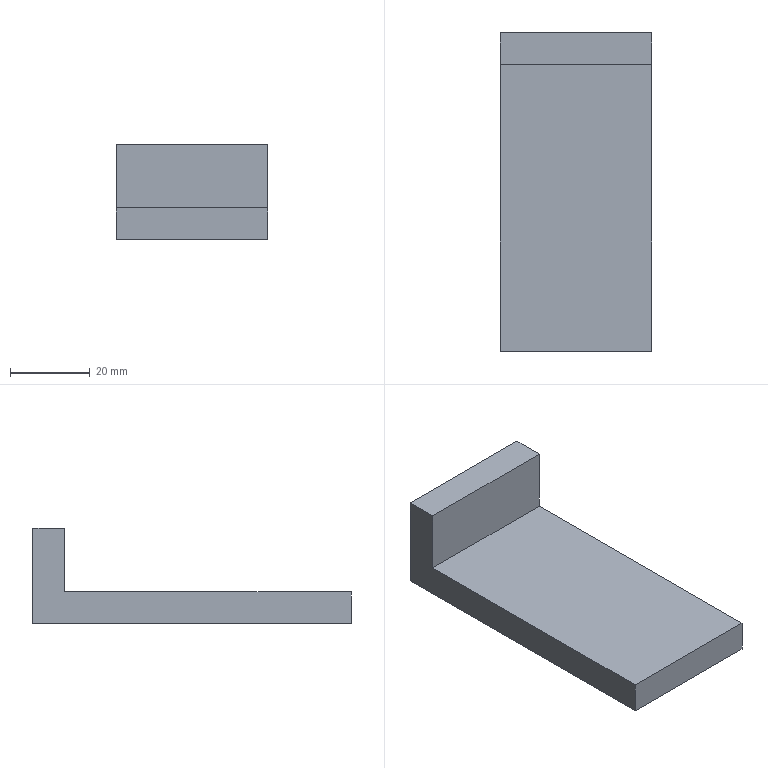Part | SolidWorks | features Extrusion 1, ICE 1 | 1 solid | 8 faces | box 38 x 80 x 24 mm | volume 29184 mm3 | plane 8
STEP:
#1=CARTESIAN_POINT('',(-19.,32.,4.));
#2=VERTEX_POINT('',#1);
#3=CARTESIAN_POINT('',(19.,32.,4.));
#4=VERTEX_POINT('',#3);
#5=CARTESIAN_POINT('',(-19.,32.,4.));
#6=DIRECTION('',(1.,0.,0.));
#7=VECTOR('',#6,1000.);
#8=LINE('',#5,#7);
#9=EDGE_CURVE('',#2,#4,#8,.T.);
#10=ORIENTED_EDGE('',*,*,#9,.F.);
#11=CARTESIAN_POINT('',(-19.,-40.,4.));
#12=VERTEX_POINT('',#11);
#13=CARTESIAN_POINT('',(-19.,-40.,4.));
#14=DIRECTION('',(0.,-1.,0.));
#15=VECTOR('',#14,1000.);
#16=LINE('',#13,#15);
#17=EDGE_CURVE('',#2,#12,#16,.T.);
#18=ORIENTED_EDGE('',*,*,#17,.T.);
#19=CARTESIAN_POINT('',(19.,-40.,4.));
#20=VERTEX_POINT('',#19);
#21=CARTESIAN_POINT('',(-19.,-40.,4.));
#22=DIRECTION('',(1.,0.,0.));
#23=VECTOR('',#22,1000.);
#24=LINE('',#21,#23);
#25=EDGE_CURVE('',#12,#20,#24,.T.);
#26=ORIENTED_EDGE('',*,*,#25,.T.);
#27=CARTESIAN_POINT('',(19.,-40.,4.));
#28=DIRECTION('',(0.,1.,0.));
#29=VECTOR('',#28,1000.);
#30=LINE('',#27,#29);
#31=EDGE_CURVE('',#20,#4,#30,.T.);
#32=ORIENTED_EDGE('',*,*,#31,.T.);
#33=EDGE_LOOP('',(#10,#18,#26,#32));
#34=FACE_OUTER_BOUND('',#33,.T.);
#35=CARTESIAN_POINT('',(0.,0.,4.));
#36=DIRECTION('',(0.,0.,-1.));
#37=DIRECTION('',(-1.,0.,0.));
#38=AXIS2_PLACEMENT_3D('',#35,#36,#37);
#39=PLANE('',#38);
#40=ADVANCED_FACE('',(#34),#39,.F.);
#41=CARTESIAN_POINT('',(19.,-40.,-4.));
#42=VERTEX_POINT('',#41);
#43=CARTESIAN_POINT('',(19.,40.,-4.));
#44=VERTEX_POINT('',#43);
#45=CARTESIAN_POINT('',(19.,-40.,-4.));
#46=DIRECTION('',(0.,1.,0.));
#47=VECTOR('',#46,1000.);
#48=LINE('',#45,#47);
#49=EDGE_CURVE('',#42,#44,#48,.T.);
#50=ORIENTED_EDGE('',*,*,#49,.T.);
#51=CARTESIAN_POINT('',(19.,40.,20.));
#52=VERTEX_POINT('',#51);
#53=CARTESIAN_POINT('',(19.,40.,4.));
#54=DIRECTION('',(0.,0.,-1.));
#55=VECTOR('',#54,1000.);
#56=LINE('',#53,#55);
#57=EDGE_CURVE('',#52,#44,#56,.T.);
#58=ORIENTED_EDGE('',*,*,#57,.F.);
#59=CARTESIAN_POINT('',(19.,32.,20.));
#60=VERTEX_POINT('',#59);
#61=CARTESIAN_POINT('',(19.,40.,20.));
#62=DIRECTION('',(0.,1.,0.));
#63=VECTOR('',#62,1000.);
#64=LINE('',#61,#63);
#65=EDGE_CURVE('',#60,#52,#64,.T.);
#66=ORIENTED_EDGE('',*,*,#65,.F.);
#67=CARTESIAN_POINT('',(19.,32.,20.));
#68=DIRECTION('',(0.,0.,-1.));
#69=VECTOR('',#68,1000.);
#70=LINE('',#67,#69);
#71=EDGE_CURVE('',#60,#4,#70,.T.);
#72=ORIENTED_EDGE('',*,*,#71,.T.);
#73=ORIENTED_EDGE('',*,*,#31,.F.);
#74=CARTESIAN_POINT('',(19.,-40.,4.));
#75=DIRECTION('',(0.,0.,-1.));
#76=VECTOR('',#75,1000.);
#77=LINE('',#74,#76);
#78=EDGE_CURVE('',#20,#42,#77,.T.);
#79=ORIENTED_EDGE('',*,*,#78,.T.);
#80=EDGE_LOOP('',(#50,#58,#66,#72,#73,#79));
#81=FACE_OUTER_BOUND('',#80,.T.);
#82=CARTESIAN_POINT('',(19.,-40.,4.));
#83=DIRECTION('',(-1.,0.,0.));
#84=DIRECTION('',(0.,0.,1.));
#85=AXIS2_PLACEMENT_3D('',#82,#83,#84);
#86=PLANE('',#85);
#87=ADVANCED_FACE('',(#81),#86,.F.);
#88=CARTESIAN_POINT('',(-19.,40.,-4.));
#89=VERTEX_POINT('',#88);
#90=CARTESIAN_POINT('',(-19.,40.,-4.));
#91=DIRECTION('',(-1.,0.,0.));
#92=VECTOR('',#91,1000.);
#93=LINE('',#90,#92);
#94=EDGE_CURVE('',#44,#89,#93,.T.);
#95=ORIENTED_EDGE('',*,*,#94,.T.);
#96=CARTESIAN_POINT('',(-19.,40.,20.));
#97=VERTEX_POINT('',#96);
#98=CARTESIAN_POINT('',(-19.,40.,4.));
#99=DIRECTION('',(0.,0.,-1.));
#100=VECTOR('',#99,1000.);
#101=LINE('',#98,#100);
#102=EDGE_CURVE('',#97,#89,#101,.T.);
#103=ORIENTED_EDGE('',*,*,#102,.F.);
#104=CARTESIAN_POINT('',(-19.,40.,20.));
#105=DIRECTION('',(-1.,0.,0.));
#106=VECTOR('',#105,1000.);
#107=LINE('',#104,#106);
#108=EDGE_CURVE('',#52,#97,#107,.T.);
#109=ORIENTED_EDGE('',*,*,#108,.F.);
#110=ORIENTED_EDGE('',*,*,#57,.T.);
#111=EDGE_LOOP('',(#95,#103,#109,#110));
#112=FACE_OUTER_BOUND('',#111,.T.);
#113=CARTESIAN_POINT('',(-19.,40.,4.));
#114=DIRECTION('',(0.,-1.,0.));
#115=DIRECTION('',(0.,0.,-1.));
#116=AXIS2_PLACEMENT_3D('',#113,#114,#115);
#117=PLANE('',#116);
#118=ADVANCED_FACE('',(#112),#117,.F.);
#119=CARTESIAN_POINT('',(-19.,-40.,-4.));
#120=VERTEX_POINT('',#119);
#121=CARTESIAN_POINT('',(-19.,-40.,-4.));
#122=DIRECTION('',(0.,-1.,0.));
#123=VECTOR('',#122,1000.);
#124=LINE('',#121,#123);
#125=EDGE_CURVE('',#89,#120,#124,.T.);
#126=ORIENTED_EDGE('',*,*,#125,.T.);
#127=CARTESIAN_POINT('',(-19.,-40.,4.));
#128=DIRECTION('',(0.,0.,-1.));
#129=VECTOR('',#128,1000.);
#130=LINE('',#127,#129);
#131=EDGE_CURVE('',#12,#120,#130,.T.);
#132=ORIENTED_EDGE('',*,*,#131,.F.);
#133=ORIENTED_EDGE('',*,*,#17,.F.);
#134=CARTESIAN_POINT('',(-19.,32.,20.));
#135=VERTEX_POINT('',#134);
#136=CARTESIAN_POINT('',(-19.,32.,20.));
#137=DIRECTION('',(0.,0.,-1.));
#138=VECTOR('',#137,1000.);
#139=LINE('',#136,#138);
#140=EDGE_CURVE('',#135,#2,#139,.T.);
#141=ORIENTED_EDGE('',*,*,#140,.F.);
#142=CARTESIAN_POINT('',(-19.,40.,20.));
#143=DIRECTION('',(0.,-1.,0.));
#144=VECTOR('',#143,1000.);
#145=LINE('',#142,#144);
#146=EDGE_CURVE('',#97,#135,#145,.T.);
#147=ORIENTED_EDGE('',*,*,#146,.F.);
#148=ORIENTED_EDGE('',*,*,#102,.T.);
#149=EDGE_LOOP('',(#126,#132,#133,#141,#147,#148));
#150=FACE_OUTER_BOUND('',#149,.T.);
#151=CARTESIAN_POINT('',(-19.,-40.,4.));
#152=DIRECTION('',(1.,0.,0.));
#153=DIRECTION('',(0.,0.,-1.));
#154=AXIS2_PLACEMENT_3D('',#151,#152,#153);
#155=PLANE('',#154);
#156=ADVANCED_FACE('',(#150),#155,.F.);
#157=CARTESIAN_POINT('',(-19.,-40.,-4.));
#158=DIRECTION('',(1.,0.,0.));
#159=VECTOR('',#158,1000.);
#160=LINE('',#157,#159);
#161=EDGE_CURVE('',#120,#42,#160,.T.);
#162=ORIENTED_EDGE('',*,*,#161,.T.);
#163=ORIENTED_EDGE('',*,*,#78,.F.);
#164=ORIENTED_EDGE('',*,*,#25,.F.);
#165=ORIENTED_EDGE('',*,*,#131,.T.);
#166=EDGE_LOOP('',(#162,#163,#164,#165));
#167=FACE_OUTER_BOUND('',#166,.T.);
#168=CARTESIAN_POINT('',(-19.,-40.,4.));
#169=DIRECTION('',(0.,1.,0.));
#170=DIRECTION('',(0.,0.,1.));
#171=AXIS2_PLACEMENT_3D('',#168,#169,#170);
#172=PLANE('',#171);
#173=ADVANCED_FACE('',(#167),#172,.F.);
#174=ORIENTED_EDGE('',*,*,#49,.F.);
#175=ORIENTED_EDGE('',*,*,#161,.F.);
#176=ORIENTED_EDGE('',*,*,#125,.F.);
#177=ORIENTED_EDGE('',*,*,#94,.F.);
#178=EDGE_LOOP('',(#174,#175,#176,#177));
#179=FACE_OUTER_BOUND('',#178,.T.);
#180=CARTESIAN_POINT('',(0.,0.,-4.));
#181=DIRECTION('',(0.,0.,-1.));
#182=DIRECTION('',(-1.,0.,0.));
#183=AXIS2_PLACEMENT_3D('',#180,#181,#182);
#184=PLANE('',#183);
#185=ADVANCED_FACE('',(#179),#184,.T.);
#186=ORIENTED_EDGE('',*,*,#9,.T.);
#187=ORIENTED_EDGE('',*,*,#71,.F.);
#188=CARTESIAN_POINT('',(-19.,32.,20.));
#189=DIRECTION('',(1.,0.,0.));
#190=VECTOR('',#189,1000.);
#191=LINE('',#188,#190);
#192=EDGE_CURVE('',#135,#60,#191,.T.);
#193=ORIENTED_EDGE('',*,*,#192,.F.);
#194=ORIENTED_EDGE('',*,*,#140,.T.);
#195=EDGE_LOOP('',(#186,#187,#193,#194));
#196=FACE_OUTER_BOUND('',#195,.T.);
#197=CARTESIAN_POINT('',(-19.,32.,20.));
#198=DIRECTION('',(0.,1.,0.));
#199=DIRECTION('',(0.,0.,1.));
#200=AXIS2_PLACEMENT_3D('',#197,#198,#199);
#201=PLANE('',#200);
#202=ADVANCED_FACE('',(#196),#201,.F.);
#203=ORIENTED_EDGE('',*,*,#146,.T.);
#204=ORIENTED_EDGE('',*,*,#192,.T.);
#205=ORIENTED_EDGE('',*,*,#65,.T.);
#206=ORIENTED_EDGE('',*,*,#108,.T.);
#207=EDGE_LOOP('',(#203,#204,#205,#206));
#208=FACE_OUTER_BOUND('',#207,.T.);
#209=CARTESIAN_POINT('',(0.,0.,20.));
#210=DIRECTION('',(0.,0.,1.));
#211=DIRECTION('',(1.,0.,0.));
#212=AXIS2_PLACEMENT_3D('',#209,#210,#211);
#213=PLANE('',#212);
#214=ADVANCED_FACE('',(#208),#213,.T.);
#215=CLOSED_SHELL('',(#40,#87,#118,#156,#173,#185,#202,#214));
#216=MANIFOLD_SOLID_BREP('',#215);
#217=CARTESIAN_POINT('',(0.,0.,0.));
#218=DIRECTION('',(0.,0.,1.));
#219=DIRECTION('',(1.,0.,0.));
#220=AXIS2_PLACEMENT_3D('',#217,#218,#219);
#221=(LENGTH_UNIT()NAMED_UNIT(*)SI_UNIT(.MILLI.,.METRE.));
#222=UNCERTAINTY_MEASURE_WITH_UNIT(LENGTH_MEASURE(0.00001),#221,'','');
#223=(NAMED_UNIT(*)PLANE_ANGLE_UNIT()SI_UNIT($,.RADIAN.));
#224=(NAMED_UNIT(*)SI_UNIT($,.STERADIAN.)SOLID_ANGLE_UNIT());
#225=(GEOMETRIC_REPRESENTATION_CONTEXT(3)GLOBAL_UNCERTAINTY_ASSIGNED_CONTEXT((#222))GLOBAL_UNIT_ASSIGNED_CONTEXT((#221,#223,#224))REPRESENTATION_CONTEXT('',''));
#226=ADVANCED_BREP_SHAPE_REPRESENTATION('',(#216,#220),#225);